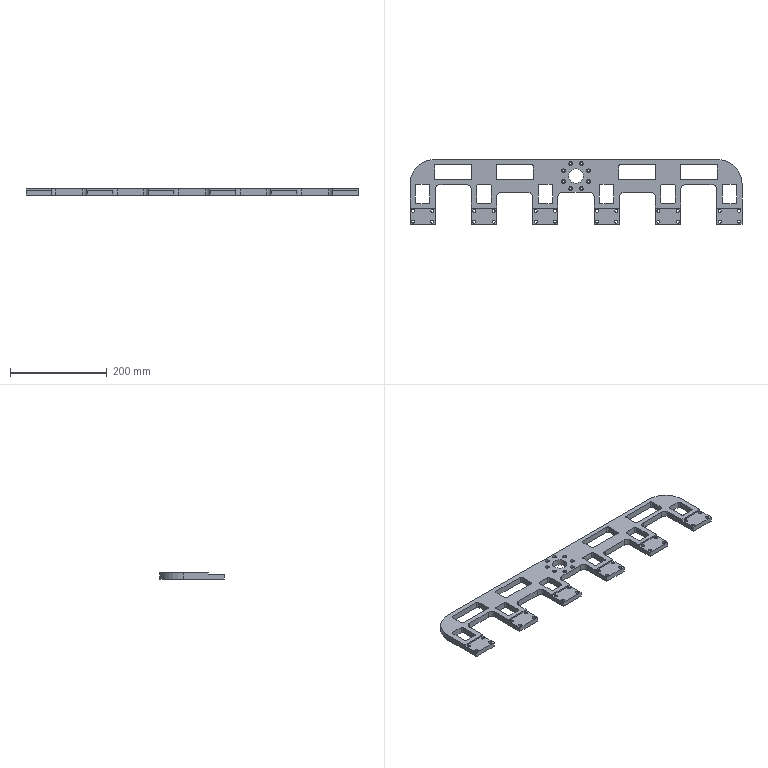NC program | NX | posted with a generic post | part box 687 x 134 x 13 mm
Lines 9027 to 9954 of 9954:
(PLANAR_MILL_COPY_1 , TOOL : D6A45)
N17998 T07 M6
N18000 G54
N18002 G17 G0 G90 X331.1 Y-4.866 S9500 M3
N18004 G43 Z30. H7
N18006 Z0.
N18008 G94 G1 Z-1. F1400.
N18010 G3 X331.6 Y-4. R1.
N18012 G1 Y13.
N18014 G3 X329.5 Y15.1 R2.1
N18016 G1 X305.5
N18018 G3 X303.4 Y13. R2.1
N18020 G1 Y-21.
N18022 G3 X305.5 Y-23.1 R2.1
N18024 G1 X329.5
N18026 G3 X331.6 Y-21. R2.1
N18028 G1 Y-4.
N18030 G3 X331.1 Y-3.134 R1.
N18032 G1 Z0.
N18034 G0 Z30.
N18036 X254.866 Y55.6
N18038 Z0.
N18040 G1 Z-1.
N18042 G3 X254. Y56.1 R1.
N18044 G1 X218.5
N18046 G3 X216.4 Y54. R2.1
N18048 G1 Y28.
N18050 G3 X218.5 Y25.9 R2.1
N18052 G1 X289.5
N18054 G3 X291.6 Y28. R2.1
N18056 G1 Y54.
N18058 G3 X289.5 Y56.1 R2.1
N18060 G1 X254.
N18062 G3 X253.134 Y55.6 R1.
N18064 G1 Z0.
N18066 G0 Z30.
N18068 X204.1 Y-4.866
N18070 Z0.
N18072 G1 Z-1.
N18074 G3 X204.6 Y-4. R1.
N18076 G1 Y13.
N18078 G3 X202.5 Y15.1 R2.1
N18080 G1 X178.5
N18082 G3 X176.4 Y13. R2.1
N18084 G1 Y-21.
N18086 G3 X178.5 Y-23.1 R2.1
N18088 G1 X202.5
N18090 G3 X204.6 Y-21. R2.1
N18092 G1 Y-4.
N18094 G3 X204.1 Y-3.134 R1.
N18096 G1 Z0.
N18098 G0 Z30.
N18100 X127.866 Y55.6
N18102 Z0.
N18104 G1 Z-1.
N18106 G3 X127. Y56.1 R1.
N18108 G1 X91.5
N18110 G3 X89.4 Y54. R2.1
N18112 G1 Y28.
N18114 G3 X91.5 Y25.9 R2.1
N18116 G1 X162.5
N18118 G3 X164.6 Y28. R2.1
N18120 G1 Y54.
N18122 G3 X162.5 Y56.1 R2.1
N18124 G1 X127.
N18126 G3 X126.134 Y55.6 R1.
N18128 G1 Z0.
N18130 G0 Z30.
N18132 X77.1 Y-4.866
N18134 Z0.
N18136 G1 Z-1.
N18138 G3 X77.6 Y-4. R1.
N18140 G1 Y13.
N18142 G3 X75.5 Y15.1 R2.1
N18144 G1 X51.5
N18146 G3 X49.4 Y13. R2.1
N18148 G1 Y-21.
N18150 G3 X51.5 Y-23.1 R2.1
N18152 G1 X75.5
N18154 G3 X77.6 Y-21. R2.1
N18156 G1 Y-4.
N18158 G3 X77.1 Y-3.134 R1.
N18160 G1 Z0.
N18162 G0 Z30.
N18164 X0.866 Y46.6
N18166 Z0.
N18168 G1 Z-1.
N18170 G3 X0. Y47.1 R1.
N18172 X-14.1 Y33. R14.1
N18174 X0. Y47.1 R-14.1
N18176 X-0.866 Y46.6 R1.
N18178 G1 Z0.
N18180 G0 Z30.
N18182 Y68.4
N18184 Z0.
N18186 G1 Z-1.
N18188 G3 X0. Y67.9 R1.
N18190 G1 X293.5
N18192 G2 X344.4 Y17. R50.9
N18194 G1 Y-33.4
N18196 G2 X343.5 Y-34.3 R0.9
N18198 G1 X291.5
N18200 G2 X290.6 Y-33.4 R0.9
N18202 G1 Y5.
N18204 G3 X281.5 Y14.1 R9.1
N18206 G1 X226.5
N18208 G3 X217.4 Y5. R9.1
N18210 G1 Y-33.4
N18212 G2 X216.5 Y-34.3 R0.9
N18214 G1 X164.5
N18216 G2 X163.6 Y-33.4 R0.9
N18218 G1 Y-10.95
N18220 G3 X154.5 Y-1.85 R9.1
N18222 G1 X99.5
N18224 G3 X90.4 Y-10.95 R9.1
N18226 G1 Y-33.4
N18228 G2 X89.5 Y-34.3 R0.9
N18230 G1 X37.5
N18232 G2 X36.6 Y-33.4 R0.9
N18234 G1 Y-10.95
N18236 G3 X27.5 Y-1.85 R9.1
N18238 G1 X-27.5
N18240 G3 X-36.6 Y-10.95 R9.1
N18242 G1 Y-33.4
N18244 G2 X-37.5 Y-34.3 R0.9
N18246 G1 X-89.5
N18248 G2 X-90.4 Y-33.4 R0.9
N18250 G1 Y-10.95
N18252 G3 X-99.5 Y-1.85 R9.1
N18254 G1 X-154.5
N18256 G3 X-163.6 Y-10.95 R9.1
N18258 G1 Y-33.4
N18260 G2 X-164.5 Y-34.3 R0.9
N18262 G1 X-216.5
N18264 G2 X-217.4 Y-33.4 R0.9
N18266 G1 Y5.
N18268 G3 X-226.5 Y14.1 R9.1
N18270 G1 X-281.5
N18272 G3 X-290.6 Y5. R9.1
N18274 G1 Y-33.4
N18276 G2 X-291.5 Y-34.3 R0.9
N18278 G1 X-343.5
N18280 G2 X-344.4 Y-33.4 R0.9
N18282 G1 Y17.
N18284 G2 X-293.5 Y67.9 R50.9
N18286 G1 X0.
N18288 G3 X0.866 Y68.4 R1.
N18290 G1 Z0.
N18292 G0 Z30.
N18294 X-49.9 Y-4.866
N18296 Z0.
N18298 G1 Z-1.
N18300 G3 X-49.4 Y-4. R1.
N18302 G1 Y13.
N18304 G3 X-51.5 Y15.1 R2.1
N18306 G1 X-75.5
N18308 G3 X-77.6 Y13. R2.1
N18310 G1 Y-21.
N18312 G3 X-75.5 Y-23.1 R2.1
N18314 G1 X-51.5
N18316 G3 X-49.4 Y-21. R2.1
N18318 G1 Y-4.
N18320 G3 X-49.9 Y-3.134 R1.
N18322 G1 Z0.
N18324 G0 Z30.
N18326 X-126.134 Y55.6
N18328 Z0.
N18330 G1 Z-1.
N18332 G3 X-127. Y56.1 R1.
N18334 G1 X-162.5
N18336 G3 X-164.6 Y54. R2.1
N18338 G1 Y28.
N18340 G3 X-162.5 Y25.9 R2.1
N18342 G1 X-91.5
N18344 G3 X-89.4 Y28. R2.1
N18346 G1 Y54.
N18348 G3 X-91.5 Y56.1 R2.1
N18350 G1 X-127.
N18352 G3 X-127.866 Y55.6 R1.
N18354 G1 Z0.
N18356 G0 Z30.
N18358 X-176.9 Y-4.866
N18360 Z0.
N18362 G1 Z-1.
N18364 G3 X-176.4 Y-4. R1.
N18366 G1 Y13.
N18368 G3 X-178.5 Y15.1 R2.1
N18370 G1 X-202.5
N18372 G3 X-204.6 Y13. R2.1
N18374 G1 Y-21.
N18376 G3 X-202.5 Y-23.1 R2.1
N18378 G1 X-178.5
N18380 G3 X-176.4 Y-21. R2.1
N18382 G1 Y-4.
N18384 G3 X-176.9 Y-3.134 R1.
N18386 G1 Z0.
N18388 G0 Z30.
N18390 X-253.134 Y55.6
N18392 Z0.
N18394 G1 Z-1.
N18396 G3 X-254. Y56.1 R1.
N18398 G1 X-289.5
N18400 G3 X-291.6 Y54. R2.1
N18402 G1 Y28.
N18404 G3 X-289.5 Y25.9 R2.1
N18406 G1 X-218.5
N18408 G3 X-216.4 Y28. R2.1
N18410 G1 Y54.
N18412 G3 X-218.5 Y56.1 R2.1
N18414 G1 X-254.
N18416 G3 X-254.866 Y55.6 R1.
N18418 G1 Z0.
N18420 G0 Z30.
N18422 X-331.1 Y-3.134
N18424 Z0.
N18426 G1 Z-1.
N18428 G3 X-331.6 Y-4. R1.
N18430 G1 Y-21.
N18432 G3 X-329.5 Y-23.1 R2.1
N18434 G1 X-305.5
N18436 G3 X-303.4 Y-21. R2.1
N18438 G1 Y13.
N18440 G3 X-305.5 Y15.1 R2.1
N18442 G1 X-329.5
N18444 G3 X-331.6 Y13. R2.1
N18446 G1 Y-4.
N18448 G3 X-331.1 Y-4.866 R1.
N18450 G1 Z0.
N18452 G0 Z30.
(PLANAR_MILL_COPY_COPY , TOOL : D6A45)
N18454 X-337.507 Y-38.1
N18456 Z-3.
N18458 G1 Z-4.
N18460 Y-37.056
N18462 G3 X-337.982 Y-36.9 R0.5
N18464 X-337.018 Y-36.9 R-2.35
N18466 X-337.493 Y-37.056 R0.5
N18468 G1 Y-38.1
N18470 Z-3.
N18472 G0 Z30.
N18474 X-337.988 Y-62.242
N18476 Z-3.
N18478 G1 Z-4.
N18480 X-338.366 Y-63.05
N18482 G3 X-337.5 Y-63.55 R1.
N18484 X-335.15 Y-61.2 R2.35
N18486 X-337.5 Y-63.55 R-2.35
N18488 X-336.634 Y-63.05 R1.
N18490 G1 X-337.012 Y-62.242
N18492 Z-3.
N18494 G0 Z30.
N18496 X-297.988
N18498 Z-3.
N18500 G1 Z-4.
N18502 X-298.366 Y-63.05
N18504 G3 X-297.5 Y-63.55 R1.
N18506 X-295.15 Y-61.2 R2.35
N18508 X-297.5 Y-63.55 R-2.35
N18510 X-296.634 Y-63.05 R1.
N18512 G1 X-297.012 Y-62.242
N18514 Z-3.
N18516 G0 Z30.
N18518 X-297.507 Y-38.1
N18520 Z-3.
N18522 G1 Z-4.
N18524 Y-37.056
N18526 G3 X-297.982 Y-36.9 R0.5
N18528 X-297.018 Y-36.9 R-2.35
N18530 X-297.493 Y-37.056 R0.5
N18532 G1 Y-38.1
N18534 Z-3.
N18536 G0 Z30.
N18538 X-210.507
N18540 Z-3.
N18542 G1 Z-4.
N18544 Y-37.056
N18546 G3 X-210.982 Y-36.9 R0.5
N18548 X-210.018 Y-36.9 R-2.35
N18550 X-210.493 Y-37.056 R0.5
N18552 G1 Y-38.1
N18554 Z-3.
N18556 G0 Z30.
N18558 X-210.988 Y-62.242
N18560 Z-3.
N18562 G1 Z-4.
N18564 X-211.366 Y-63.05
N18566 G3 X-210.5 Y-63.55 R1.
N18568 X-208.15 Y-61.2 R2.35
N18570 X-210.5 Y-63.55 R-2.35
N18572 X-209.634 Y-63.05 R1.
N18574 G1 X-210.012 Y-62.242
N18576 Z-3.
N18578 G0 Z30.
N18580 X-170.988
N18582 Z-3.
N18584 G1 Z-4.
N18586 X-171.366 Y-63.05
N18588 G3 X-170.5 Y-63.55 R1.
N18590 X-168.15 Y-61.2 R2.35
N18592 X-170.5 Y-63.55 R-2.35
N18594 X-169.634 Y-63.05 R1.
N18596 G1 X-170.012 Y-62.242
N18598 Z-3.
N18600 G0 Z30.
N18602 X-170.507 Y-38.1
N18604 Z-3.
N18606 G1 Z-4.
N18608 Y-37.056
N18610 G3 X-170.982 Y-36.9 R0.5
N18612 X-170.018 Y-36.9 R-2.35
N18614 X-170.493 Y-37.056 R0.5
N18616 G1 Y-38.1
N18618 Z-3.
N18620 G0 Z30.
N18622 X-83.507
N18624 Z-3.
N18626 G1 Z-4.
N18628 Y-37.056
N18630 G3 X-83.982 Y-36.9 R0.5
N18632 X-83.018 Y-36.9 R-2.35
N18634 X-83.493 Y-37.056 R0.5
N18636 G1 Y-38.1
N18638 Z-3.
N18640 G0 Z30.
N18642 X-83.988 Y-62.242
N18644 Z-3.
N18646 G1 Z-4.
N18648 X-84.366 Y-63.05
N18650 G3 X-83.5 Y-63.55 R1.
N18652 X-81.15 Y-61.2 R2.35
N18654 X-83.5 Y-63.55 R-2.35
N18656 X-82.634 Y-63.05 R1.
N18658 G1 X-83.012 Y-62.242
N18660 Z-3.
N18662 G0 Z30.
N18664 X-43.988
N18666 Z-3.
N18668 G1 Z-4.
N18670 X-44.366 Y-63.05
N18672 G3 X-43.5 Y-63.55 R1.
N18674 X-41.15 Y-61.2 R2.35
N18676 X-43.5 Y-63.55 R-2.35
N18678 X-42.634 Y-63.05 R1.
N18680 G1 X-43.012 Y-62.242
N18682 Z-3.
N18684 G0 Z30.
N18686 X-43.507 Y-38.1
N18688 Z-3.
N18690 G1 Z-4.
N18692 Y-37.056
N18694 G3 X-43.982 Y-36.9 R0.5
N18696 X-43.018 Y-36.9 R-2.35
N18698 X-43.493 Y-37.056 R0.5
N18700 G1 Y-38.1
N18702 Z-3.
N18704 G0 Z30.
N18706 X-35.187 Y-37.492
N18708 Z-3.
N18710 G1 Z-4.
N18712 X-35.635 Y-37.043
N18714 G3 X-36.6 Y-36.782 R1.
N18716 G1 Y-66.9
N18718 G2 X-37.6 Y-67.9 R1.
N18720 G1 X-89.4
N18722 G2 X-90.4 Y-66.9 R1.
N18724 G1 Y-36.782
N18726 G3 X-91.365 Y-37.043 R1.
N18728 G1 X-91.813 Y-37.492
N18730 Z-3.
N18732 G0 Z30.
N18734 X-162.187
N18736 Z-3.
N18738 G1 Z-4.
N18740 X-162.635 Y-37.043
N18742 G3 X-163.6 Y-36.782 R1.
N18744 G1 Y-66.9
N18746 G2 X-164.6 Y-67.9 R1.
N18748 G1 X-216.4
N18750 G2 X-217.4 Y-66.9 R1.
N18752 G1 Y-36.782
N18754 G3 X-218.365 Y-37.043 R1.
N18756 G1 X-218.813 Y-37.492
N18758 Z-3.
N18760 G0 Z30.
N18762 X-289.187
N18764 Z-3.
N18766 G1 Z-4.
N18768 X-289.635 Y-37.043
N18770 G3 X-290.6 Y-36.782 R1.
N18772 G1 Y-66.9
N18774 G2 X-291.6 Y-67.9 R1.
N18776 G1 X-343.4
N18778 G2 X-344.4 Y-66.9 R1.
N18780 G1 Y-36.782
N18782 G3 X-345.365 Y-37.043 R1.
N18784 G1 X-345.813 Y-37.492
N18786 Z-3.
N18788 G0 Z30.
N18790 X345.813
N18792 Z-3.
N18794 G1 Z-4.
N18796 X345.365 Y-37.043
N18798 G3 X344.4 Y-36.782 R1.
N18800 G1 Y-66.9
N18802 G2 X343.4 Y-67.9 R1.
N18804 G1 X291.6
N18806 G2 X290.6 Y-66.9 R1.
N18808 G1 Y-36.782
N18810 G3 X289.635 Y-37.043 R1.
N18812 G1 X289.187 Y-37.492
N18814 Z-3.
N18816 G0 Z30.
N18818 X218.813
N18820 Z-3.
N18822 G1 Z-4.
N18824 X218.365 Y-37.043
N18826 G3 X217.4 Y-36.782 R1.
N18828 G1 Y-66.9
N18830 G2 X216.4 Y-67.9 R1.
N18832 G1 X164.6
N18834 G2 X163.6 Y-66.9 R1.
N18836 G1 Y-36.782
N18838 G3 X162.635 Y-37.043 R1.
N18840 G1 X162.187 Y-37.492
N18842 Z-3.
N18844 G0 Z30.
N18846 X91.813
N18848 Z-3.
N18850 G1 Z-4.
N18852 X91.365 Y-37.043
N18854 G3 X90.4 Y-36.782 R1.
N18856 G1 Y-66.9
N18858 G2 X89.4 Y-67.9 R1.
N18860 G1 X37.6
N18862 G2 X36.6 Y-66.9 R1.
N18864 G1 Y-36.782
N18866 G3 X35.635 Y-37.043 R1.
N18868 G1 X35.187 Y-37.492
N18870 Z-3.
N18872 G0 Z30.
N18874 X43.493 Y-38.1
N18876 Z-3.
N18878 G1 Z-4.
N18880 Y-37.056
N18882 G3 X43.018 Y-36.9 R0.5
N18884 X43.982 Y-36.9 R-2.35
N18886 X43.507 Y-37.056 R0.5
N18888 G1 Y-38.1
N18890 Z-3.
N18892 G0 Z30.
N18894 X43.012 Y-62.242
N18896 Z-3.
N18898 G1 Z-4.
N18900 X42.634 Y-63.05
N18902 G3 X43.5 Y-63.55 R1.
N18904 X45.85 Y-61.2 R2.35
N18906 X43.5 Y-63.55 R-2.35
N18908 X44.366 Y-63.05 R1.
N18910 G1 X43.988 Y-62.242
N18912 Z-3.
N18914 G0 Z30.
N18916 X83.012
N18918 Z-3.
N18920 G1 Z-4.
N18922 X82.634 Y-63.05
N18924 G3 X83.5 Y-63.55 R1.
N18926 X85.85 Y-61.2 R2.35
N18928 X83.5 Y-63.55 R-2.35
N18930 X84.366 Y-63.05 R1.
N18932 G1 X83.988 Y-62.242
N18934 Z-3.
N18936 G0 Z30.
N18938 X83.493 Y-38.1
N18940 Z-3.
N18942 G1 Z-4.
N18944 Y-37.056
N18946 G3 X83.018 Y-36.9 R0.5
N18948 X83.982 Y-36.9 R-2.35
N18950 X83.507 Y-37.056 R0.5
N18952 G1 Y-38.1
N18954 Z-3.
N18956 G0 Z30.
N18958 X170.493
N18960 Z-3.
N18962 G1 Z-4.
N18964 Y-37.056
N18966 G3 X170.018 Y-36.9 R0.5
N18968 X170.982 Y-36.9 R-2.35
N18970 X170.507 Y-37.056 R0.5
N18972 G1 Y-38.1
N18974 Z-3.
N18976 G0 Z30.
N18978 X170.012 Y-62.242
N18980 Z-3.
N18982 G1 Z-4.
N18984 X169.634 Y-63.05
N18986 G3 X170.5 Y-63.55 R1.
N18988 X172.85 Y-61.2 R2.35
N18990 X170.5 Y-63.55 R-2.35
N18992 X171.366 Y-63.05 R1.
N18994 G1 X170.988 Y-62.242
N18996 Z-3.
N18998 G0 Z30.
N19000 X210.012
N19002 Z-3.
N19004 G1 Z-4.
N19006 X209.634 Y-63.05
N19008 G3 X210.5 Y-63.55 R1.
N19010 X212.85 Y-61.2 R2.35
N19012 X210.5 Y-63.55 R-2.35
N19014 X211.366 Y-63.05 R1.
N19016 G1 X210.988 Y-62.242
N19018 Z-3.
N19020 G0 Z30.
N19022 X210.493 Y-38.1
N19024 Z-3.
N19026 G1 Z-4.
N19028 Y-37.056
N19030 G3 X210.018 Y-36.9 R0.5
N19032 X210.982 Y-36.9 R-2.35
N19034 X210.507 Y-37.056 R0.5
N19036 G1 Y-38.1
N19038 Z-3.
N19040 G0 Z30.
N19042 X297.493
N19044 Z-3.
N19046 G1 Z-4.
N19048 Y-37.056
N19050 G3 X297.018 Y-36.9 R0.5
N19052 X297.982 Y-36.9 R-2.35
N19054 X297.507 Y-37.056 R0.5
N19056 G1 Y-38.1
N19058 Z-3.
N19060 G0 Z30.
N19062 X297.012 Y-62.242
N19064 Z-3.
N19066 G1 Z-4.
N19068 X296.634 Y-63.05
N19070 G3 X297.5 Y-63.55 R1.
N19072 X299.85 Y-61.2 R2.35
N19074 X297.5 Y-63.55 R-2.35
N19076 X298.366 Y-63.05 R1.
N19078 G1 X297.988 Y-62.242
N19080 Z-3.
N19082 G0 Z30.
N19084 X337.012
N19086 Z-3.
N19088 G1 Z-4.
N19090 X336.634 Y-63.05
N19092 G3 X337.5 Y-63.55 R1.
N19094 X339.85 Y-61.2 R2.35
N19096 X337.5 Y-63.55 R-2.35
N19098 X338.366 Y-63.05 R1.
N19100 G1 X337.988 Y-62.242
N19102 Z-3.
N19104 G0 Z30.
N19106 X337.493 Y-38.1
N19108 Z-3.
N19110 G1 Z-4.
N19112 Y-37.056
N19114 G3 X337.018 Y-36.9 R0.5
N19116 X337.982 Y-36.9 R-2.35
N19118 X337.507 Y-37.056 R0.5
N19120 G1 Y-38.1
N19122 Z-3.
N19124 G0 Z30.
N19126 M5
(ZLEVEL_PROFILE_COPY_3_COPY , TOOL : D10)
N19128 T10 M6
N19130 G54
N19132 G17 G0 G90 X-286.5 Y-54.524 S9500 M3
N19134 G43 Z30. H10
N19136 Z-1.
N19138 G94 G1 Y-67.316 Z-1.67 F1000.
N19140 X-286.615 Y-68.111 Z-1.713
N19142 X-286.855 Y-68.878 Z-1.755
N19144 X-287.215 Y-69.596 Z-1.797
N19146 X-287.685 Y-70.247 Z-1.839
N19148 X-288.253 Y-70.815 Z-1.881
N19150 X-288.904 Y-71.285 Z-1.923
N19152 X-289.622 Y-71.645 Z-1.965
N19154 X-290.389 Y-71.885 Z-2.007
N19156 X-291.184 Y-72. Z-2.049
N19158 X-343.816 Z-4.808
N19160 X-344.611 Y-71.885 Z-4.85
N19162 X-345.378 Y-71.645 Z-4.892
N19164 X-346.096 Y-71.285 Z-4.934
N19166 X-346.747 Y-70.815 Z-4.976
N19168 X-347.315 Y-70.247 Z-5.018
N19170 X-347.785 Y-69.596 Z-5.06
N19172 X-348.145 Y-68.878 Z-5.102
N19174 X-348.385 Y-68.111 Z-5.144
N19176 X-348.5 Y-67.316 Z-5.186
N19178 Y18.049 Z-9.66
N19180 X-348.368 Y20.953 Z-9.813
N19182 X-348.082 Y23.846 Z-9.965
N19184 X-347.645 Y26.72 Z-10.117
N19186 X-347.055 Y29.566 Z-10.27
N19188 X-346.317 Y32.378 Z-10.422
N19190 X-345.431 Y35.146 Z-10.574
N19192 X-344.4 Y37.864 Z-10.727
N19194 X-343.226 Y40.524 Z-10.879
N19196 X-341.914 Y43.118 Z-11.031
N19198 X-340.467 Y45.639 Z-11.184
N19200 X-338.889 Y48.08 Z-11.336
N19202 X-337.183 Y50.434 Z-11.488
N19204 X-335.356 Y52.695 Z-11.641
N19206 X-333.412 Y54.857 Z-11.793
N19208 X-331.357 Y56.912 Z-11.946
N19210 X-329.195 Y58.856 Z-12.098
N19212 X-326.934 Y60.683 Z-12.25
N19214 X-324.58 Y62.389 Z-12.403
N19216 X-322.139 Y63.967 Z-12.555
N19218 X-319.618 Y65.414 Z-12.707
N19220 X-317.024 Y66.726 Z-12.86
N19222 X-314.364 Y67.9 Z-13.012
N19224 X-311.646 Y68.931 Z-13.164
N19226 X-308.878 Y69.817 Z-13.317
N19228 X-306.066 Y70.555 Z-13.469
N19230 X-303.22 Y71.145 Z-13.621
N19232 X-300.346 Y71.582 Z-13.774
N19234 X-297.453 Y71.868 Z-13.926
N19236 X-294.549 Y72. Z-14.078
N19238 X-293.5 Z-14.133
N19240 X293.5 F1200.
N19242 G2 X348.5 Y17. R55.
N19244 G1 Y-67.
N19246 G2 X343.5 Y-72. R5.
N19248 G1 X291.5
N19250 G2 X286.5 Y-67. R5.
N19252 G1 Y5.
N19254 G3 X281.5 Y10. R5.
N19256 G1 X226.497
N19258 G3 X221.5 Y5. R5.
N19260 G1 Y-67.
N19262 G2 X216.5 Y-72. R5.
N19264 G1 X164.5
N19266 G2 X159.5 Y-67. R5.
N19268 G1 Y-10.95
N19270 G3 X154.5 Y-5.95 R5.
N19272 G1 X99.5
N19274 G3 X94.5 Y-10.95 R5.
N19276 G1 Y-67.
N19278 G2 X89.5 Y-72. R5.
N19280 G1 X37.5
N19282 G2 X32.5 Y-67. R5.
N19284 G1 Y-10.95
N19286 G3 X27.5 Y-5.95 R5.
N19288 G1 X-27.506
N19290 G3 X-32.5 Y-10.95 R5.
N19292 G1 Y-67.
N19294 G2 X-37.5 Y-72. R5.
N19296 G1 X-89.5
N19298 G2 X-94.5 Y-67. R5.
N19300 G1 Y-10.95
N19302 G3 X-99.5 Y-5.95 R5.
N19304 G1 X-154.494
N19306 G3 X-159.5 Y-10.95 R5.
N19308 G1 Y-67.
N19310 G2 X-164.5 Y-72. R5.
N19312 G1 X-216.5
N19314 G2 X-221.5 Y-67. R5.
N19316 G1 Y5.
N19318 G3 X-226.5 Y10. R5.
N19320 G1 X-281.495
N19322 G3 X-286.5 Y5. R5.
N19324 G1 Y-67.
N19326 G2 X-291.5 Y-72. R5.
N19328 G1 X-343.5
N19330 G2 X-348.5 Y-67. R5.
N19332 G1 Y17.
N19334 G2 X-293.5 Y72. R55.
N19336 G1 X-285.861 Z-14.267
N19338 X293.5
N19340 G2 X348.5 Y17. R55.
N19342 G1 Y-67.
N19344 G2 X343.5 Y-72. R5.
N19346 G1 X291.5
N19348 G2 X286.5 Y-67. R5.
N19350 G1 Y5.
N19352 G3 X281.5 Y10. R5.
N19354 G1 X226.497
N19356 G3 X221.5 Y5. R5.
N19358 G1 Y-67.
N19360 G2 X216.5 Y-72. R5.
N19362 G1 X164.5
N19364 G2 X159.5 Y-67. R5.
N19366 G1 Y-10.95
N19368 G3 X154.5 Y-5.95 R5.
N19370 G1 X99.5
N19372 G3 X94.5 Y-10.95 R5.
N19374 G1 Y-67.
N19376 G2 X89.5 Y-72. R5.
N19378 G1 X37.5
N19380 G2 X32.5 Y-67. R5.
N19382 G1 Y-10.95
N19384 G3 X27.5 Y-5.95 R5.
N19386 G1 X-27.506
N19388 G3 X-32.5 Y-10.95 R5.
N19390 G1 Y-67.
N19392 G2 X-37.5 Y-72. R5.
N19394 G1 X-89.5
N19396 G2 X-94.5 Y-67. R5.
N19398 G1 Y-10.95
N19400 G3 X-99.5 Y-5.95 R5.
N19402 G1 X-154.494
N19404 G3 X-159.5 Y-10.95 R5.
N19406 G1 Y-67.
N19408 G2 X-164.5 Y-72. R5.
N19410 G1 X-216.5
N19412 G2 X-221.5 Y-67. R5.
N19414 G1 Y5.
N19416 G3 X-226.5 Y10. R5.
N19418 G1 X-281.495
N19420 G3 X-286.5 Y5. R5.
N19422 G1 Y-67.
N19424 G2 X-291.5 Y-72. R5.
N19426 G1 X-343.5
N19428 G2 X-348.5 Y-67. R5.
N19430 G1 Y17.
N19432 G2 X-293.5 Y72. R55.
N19434 G1 X-285.861 Z-14.4
N19436 X293.5
N19438 G2 X348.5 Y17. R55.
N19440 G1 Y-67.
N19442 G2 X343.5 Y-72. R5.
N19444 G1 X291.5
N19446 G2 X286.5 Y-67. R5.
N19448 G1 Y5.
N19450 G3 X281.5 Y10. R5.
N19452 G1 X226.497
N19454 G3 X221.5 Y5. R5.
N19456 G1 Y-67.
N19458 G2 X216.5 Y-72. R5.
N19460 G1 X164.5
N19462 G2 X159.5 Y-67. R5.
N19464 G1 Y-10.95
N19466 G3 X154.5 Y-5.95 R5.
N19468 G1 X99.5
N19470 G3 X94.5 Y-10.95 R5.
N19472 G1 Y-67.
N19474 G2 X89.5 Y-72. R5.
N19476 G1 X37.5
N19478 G2 X32.5 Y-67. R5.
N19480 G1 Y-10.95
N19482 G3 X27.5 Y-5.95 R5.
N19484 G1 X-27.506
N19486 G3 X-32.5 Y-10.95 R5.
N19488 G1 Y-67.
N19490 G2 X-37.5 Y-72. R5.
N19492 G1 X-89.5
N19494 G2 X-94.5 Y-67. R5.
N19496 G1 Y-10.95
N19498 G3 X-99.5 Y-5.95 R5.
N19500 G1 X-154.494
N19502 G3 X-159.5 Y-10.95 R5.
N19504 G1 Y-67.
N19506 G2 X-164.5 Y-72. R5.
N19508 G1 X-216.5
N19510 G2 X-221.5 Y-67. R5.
N19512 G1 Y5.
N19514 G3 X-226.5 Y10. R5.
N19516 G1 X-281.495
N19518 G3 X-286.5 Y5. R5.
N19520 G1 Y-67.
N19522 G2 X-291.5 Y-72. R5.
N19524 G1 X-343.5
N19526 G2 X-348.5 Y-67. R5.
N19528 G1 Y17.
N19530 G2 X-293.5 Y72. R55.
N19532 G1 X-285.861 Z-14.533
N19534 X293.5
N19536 G2 X348.5 Y17. R55.
N19538 G1 Y-67.
N19540 G2 X343.5 Y-72. R5.
N19542 G1 X291.5
N19544 G2 X286.5 Y-67. R5.
N19546 G1 Y5.
N19548 G3 X281.5 Y10. R5.
N19550 G1 X226.497
N19552 G3 X221.5 Y5. R5.
N19554 G1 Y-67.
N19556 G2 X216.5 Y-72. R5.
N19558 G1 X164.5
N19560 G2 X159.5 Y-67. R5.
N19562 G1 Y-10.95
N19564 G3 X154.5 Y-5.95 R5.
N19566 G1 X99.5
N19568 G3 X94.5 Y-10.95 R5.
N19570 G1 Y-67.
N19572 G2 X89.5 Y-72. R5.
N19574 G1 X37.5
N19576 G2 X32.5 Y-67. R5.
N19578 G1 Y-10.95
N19580 G3 X27.5 Y-5.95 R5.
N19582 G1 X-27.506
N19584 G3 X-32.5 Y-10.95 R5.
N19586 G1 Y-67.
N19588 G2 X-37.5 Y-72. R5.
N19590 G1 X-89.5
N19592 G2 X-94.5 Y-67. R5.
N19594 G1 Y-10.95
N19596 G3 X-99.5 Y-5.95 R5.
N19598 G1 X-154.494
N19600 G3 X-159.5 Y-10.95 R5.
N19602 G1 Y-67.
N19604 G2 X-164.5 Y-72. R5.
N19606 G1 X-216.5
N19608 G2 X-221.5 Y-67. R5.
N19610 G1 Y5.
N19612 G3 X-226.5 Y10. R5.
N19614 G1 X-281.495
N19616 G3 X-286.5 Y5. R5.
N19618 G1 Y-67.
N19620 G2 X-291.5 Y-72. R5.
N19622 G1 X-343.5
N19624 G2 X-348.5 Y-67. R5.
N19626 G1 Y17.
N19628 G2 X-293.5 Y72. R55.
N19630 G1 X-285.861 Z-14.667
N19632 X293.5
N19634 G2 X348.5 Y17. R55.
N19636 G1 Y-67.
N19638 G2 X343.5 Y-72. R5.
N19640 G1 X291.5
N19642 G2 X286.5 Y-67. R5.
N19644 G1 Y5.
N19646 G3 X281.5 Y10. R5.
N19648 G1 X226.497
N19650 G3 X221.5 Y5. R5.
N19652 G1 Y-67.
N19654 G2 X216.5 Y-72. R5.
N19656 G1 X164.5
N19658 G2 X159.5 Y-67. R5.
N19660 G1 Y-10.95
N19662 G3 X154.5 Y-5.95 R5.
N19664 G1 X99.5
N19666 G3 X94.5 Y-10.95 R5.
N19668 G1 Y-67.
N19670 G2 X89.5 Y-72. R5.
N19672 G1 X37.5
N19674 G2 X32.5 Y-67. R5.
N19676 G1 Y-10.95
N19678 G3 X27.5 Y-5.95 R5.
N19680 G1 X-27.506
N19682 G3 X-32.5 Y-10.95 R5.
N19684 G1 Y-67.
N19686 G2 X-37.5 Y-72. R5.
N19688 G1 X-89.5
N19690 G2 X-94.5 Y-67. R5.
N19692 G1 Y-10.95
N19694 G3 X-99.5 Y-5.95 R5.
N19696 G1 X-154.494
N19698 G3 X-159.5 Y-10.95 R5.
N19700 G1 Y-67.
N19702 G2 X-164.5 Y-72. R5.
N19704 G1 X-216.5
N19706 G2 X-221.5 Y-67. R5.
N19708 G1 Y5.
N19710 G3 X-226.5 Y10. R5.
N19712 G1 X-281.495
N19714 G3 X-286.5 Y5. R5.
N19716 G1 Y-67.
N19718 G2 X-291.5 Y-72. R5.
N19720 G1 X-343.5
N19722 G2 X-348.5 Y-67. R5.
N19724 G1 Y17.
N19726 G2 X-293.5 Y72. R55.
N19728 G1 X-285.861 Z-14.8
N19730 X293.5
N19732 G2 X348.5 Y17. R55.
N19734 G1 Y-67.
N19736 G2 X343.5 Y-72. R5.
N19738 G1 X291.5
N19740 G2 X286.5 Y-67. R5.
N19742 G1 Y5.
N19744 G3 X281.5 Y10. R5.
N19746 G1 X226.497
N19748 G3 X221.5 Y5. R5.
N19750 G1 Y-67.
N19752 G2 X216.5 Y-72. R5.
N19754 G1 X164.5
N19756 G2 X159.5 Y-67. R5.
N19758 G1 Y-10.95
N19760 G3 X154.5 Y-5.95 R5.
N19762 G1 X99.5
N19764 G3 X94.5 Y-10.95 R5.
N19766 G1 Y-67.
N19768 G2 X89.5 Y-72. R5.
N19770 G1 X37.5
N19772 G2 X32.5 Y-67. R5.
N19774 G1 Y-10.95
N19776 G3 X27.5 Y-5.95 R5.
N19778 G1 X-27.506
N19780 G3 X-32.5 Y-10.95 R5.
N19782 G1 Y-67.
N19784 G2 X-37.5 Y-72. R5.
N19786 G1 X-89.5
N19788 G2 X-94.5 Y-67. R5.
N19790 G1 Y-10.95
N19792 G3 X-99.5 Y-5.95 R5.
N19794 G1 X-154.494
N19796 G3 X-159.5 Y-10.95 R5.
N19798 G1 Y-67.
N19800 G2 X-164.5 Y-72. R5.
N19802 G1 X-216.5
N19804 G2 X-221.5 Y-67. R5.
N19806 G1 Y5.
N19808 G3 X-226.5 Y10. R5.
N19810 G1 X-281.495
N19812 G3 X-286.5 Y5. R5.
N19814 G1 Y-67.
N19816 G2 X-291.5 Y-72. R5.
N19818 G1 X-343.5
N19820 G2 X-348.5 Y-67. R5.
N19822 G1 Y17.
N19824 G2 X-293.5 Y72. R55.
N19826 G1 X-285.861
N19828 Z-1.8
N19830 G0 Z30.
N19832 M5
N19834 M2